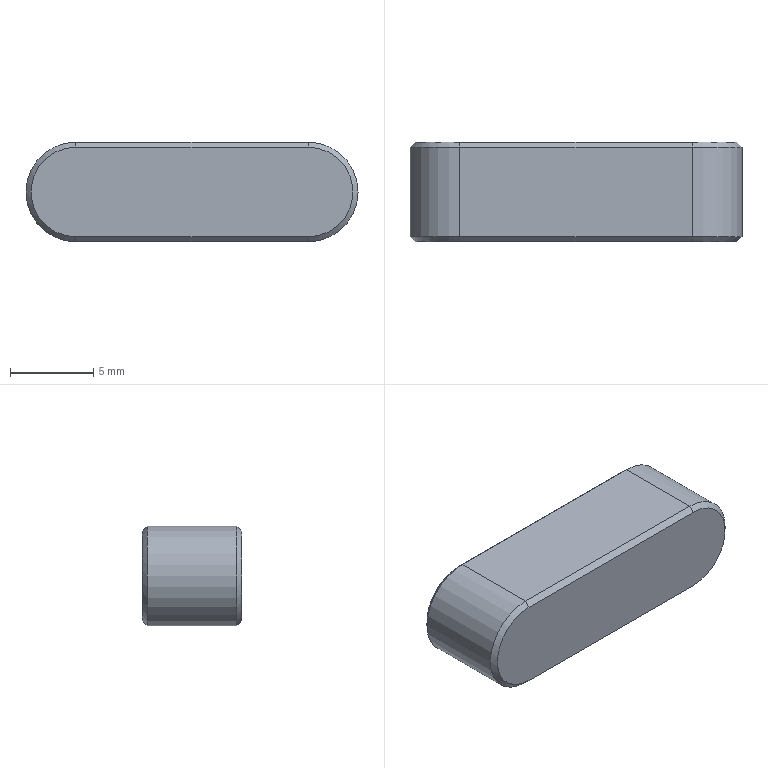Part | NX | features BREP 1 | 1 solid | 14 faces | box 20 x 6 x 6 mm | volume 669.486 mm3 | plane 8 | cone 4 | cylinder 2 | commonest cylinder face diameters 6 x2
STEP:
#1=CARTESIAN_POINT('',(-7.,5.7,3.));
#2=VERTEX_POINT('',#1);
#3=CARTESIAN_POINT('',(-7.,0.3,3.));
#4=VERTEX_POINT('',#3);
#5=CARTESIAN_POINT('',(-7.,6.,3.));
#6=DIRECTION('',(0.,-1.,0.));
#7=VECTOR('',#6,1000.);
#8=LINE('',#5,#7);
#9=EDGE_CURVE('',#2,#4,#8,.T.);
#10=ORIENTED_EDGE('',*,*,#9,.F.);
#11=CARTESIAN_POINT('',(-7.,5.7,-3.));
#12=VERTEX_POINT('',#11);
#13=CARTESIAN_POINT('',(-7.,5.7,0.));
#14=DIRECTION('',(0.,-1.,0.));
#15=DIRECTION('',(0.,0.,1.));
#16=AXIS2_PLACEMENT_3D('',#13,#14,#15);
#17=CIRCLE('',#16,3.);
#18=EDGE_CURVE('',#2,#12,#17,.T.);
#19=ORIENTED_EDGE('',*,*,#18,.T.);
#20=CARTESIAN_POINT('',(-7.,0.3,-3.));
#21=VERTEX_POINT('',#20);
#22=CARTESIAN_POINT('',(-7.,6.,-3.));
#23=DIRECTION('',(0.,-1.,0.));
#24=VECTOR('',#23,1000.);
#25=LINE('',#22,#24);
#26=EDGE_CURVE('',#12,#21,#25,.T.);
#27=ORIENTED_EDGE('',*,*,#26,.T.);
#28=CARTESIAN_POINT('',(-7.,0.3,0.));
#29=DIRECTION('',(0.,1.,0.));
#30=DIRECTION('',(0.,0.,1.));
#31=AXIS2_PLACEMENT_3D('',#28,#29,#30);
#32=CIRCLE('',#31,3.);
#33=EDGE_CURVE('',#21,#4,#32,.T.);
#34=ORIENTED_EDGE('',*,*,#33,.T.);
#35=EDGE_LOOP('',(#10,#19,#27,#34));
#36=FACE_BOUND('',#35,.T.);
#37=CARTESIAN_POINT('',(-7.,6.,0.));
#38=DIRECTION('',(0.,-1.,0.));
#39=DIRECTION('',(0.,0.,1.));
#40=AXIS2_PLACEMENT_3D('',#37,#38,#39);
#41=CYLINDRICAL_SURFACE('',#40,3.);
#42=ADVANCED_FACE('',(#36),#41,.T.);
#43=CARTESIAN_POINT('',(7.,5.7,3.));
#44=VERTEX_POINT('',#43);
#45=CARTESIAN_POINT('',(7.,0.3,3.));
#46=VERTEX_POINT('',#45);
#47=CARTESIAN_POINT('',(7.,6.,3.));
#48=DIRECTION('',(0.,-1.,0.));
#49=VECTOR('',#48,1000.);
#50=LINE('',#47,#49);
#51=EDGE_CURVE('',#44,#46,#50,.T.);
#52=ORIENTED_EDGE('',*,*,#51,.F.);
#53=CARTESIAN_POINT('',(-7.,5.7,3.));
#54=DIRECTION('',(-1.,0.,0.));
#55=VECTOR('',#54,1000.);
#56=LINE('',#53,#55);
#57=EDGE_CURVE('',#44,#2,#56,.T.);
#58=ORIENTED_EDGE('',*,*,#57,.T.);
#59=ORIENTED_EDGE('',*,*,#9,.T.);
#60=CARTESIAN_POINT('',(-7.,0.3,3.));
#61=DIRECTION('',(1.,0.,0.));
#62=VECTOR('',#61,1000.);
#63=LINE('',#60,#62);
#64=EDGE_CURVE('',#4,#46,#63,.T.);
#65=ORIENTED_EDGE('',*,*,#64,.T.);
#66=EDGE_LOOP('',(#52,#58,#59,#65));
#67=FACE_BOUND('',#66,.T.);
#68=CARTESIAN_POINT('',(-7.,6.,3.));
#69=DIRECTION('',(0.,0.,-1.));
#70=DIRECTION('',(1.,0.,0.));
#71=AXIS2_PLACEMENT_3D('',#68,#69,#70);
#72=PLANE('',#71);
#73=ADVANCED_FACE('',(#67),#72,.F.);
#74=CARTESIAN_POINT('',(7.,5.7,-3.));
#75=VERTEX_POINT('',#74);
#76=CARTESIAN_POINT('',(7.,0.3,-3.));
#77=VERTEX_POINT('',#76);
#78=CARTESIAN_POINT('',(7.,6.,-3.));
#79=DIRECTION('',(0.,-1.,0.));
#80=VECTOR('',#79,1000.);
#81=LINE('',#78,#80);
#82=EDGE_CURVE('',#75,#77,#81,.T.);
#83=ORIENTED_EDGE('',*,*,#82,.F.);
#84=CARTESIAN_POINT('',(7.,5.7,0.));
#85=DIRECTION('',(0.,-1.,0.));
#86=DIRECTION('',(0.,0.,1.));
#87=AXIS2_PLACEMENT_3D('',#84,#85,#86);
#88=CIRCLE('',#87,3.);
#89=EDGE_CURVE('',#75,#44,#88,.T.);
#90=ORIENTED_EDGE('',*,*,#89,.T.);
#91=ORIENTED_EDGE('',*,*,#51,.T.);
#92=CARTESIAN_POINT('',(7.,0.3,0.));
#93=DIRECTION('',(0.,1.,0.));
#94=DIRECTION('',(0.,0.,1.));
#95=AXIS2_PLACEMENT_3D('',#92,#93,#94);
#96=CIRCLE('',#95,3.);
#97=EDGE_CURVE('',#46,#77,#96,.T.);
#98=ORIENTED_EDGE('',*,*,#97,.T.);
#99=EDGE_LOOP('',(#83,#90,#91,#98));
#100=FACE_BOUND('',#99,.T.);
#101=CARTESIAN_POINT('',(7.,6.,0.));
#102=DIRECTION('',(0.,-1.,0.));
#103=DIRECTION('',(0.,0.,1.));
#104=AXIS2_PLACEMENT_3D('',#101,#102,#103);
#105=CYLINDRICAL_SURFACE('',#104,3.);
#106=ADVANCED_FACE('',(#100),#105,.T.);
#107=ORIENTED_EDGE('',*,*,#26,.F.);
#108=CARTESIAN_POINT('',(7.,5.7,-3.));
#109=DIRECTION('',(1.,0.,0.));
#110=VECTOR('',#109,1000.);
#111=LINE('',#108,#110);
#112=EDGE_CURVE('',#12,#75,#111,.T.);
#113=ORIENTED_EDGE('',*,*,#112,.T.);
#114=ORIENTED_EDGE('',*,*,#82,.T.);
#115=CARTESIAN_POINT('',(7.,0.3,-3.));
#116=DIRECTION('',(-1.,0.,0.));
#117=VECTOR('',#116,1000.);
#118=LINE('',#115,#117);
#119=EDGE_CURVE('',#77,#21,#118,.T.);
#120=ORIENTED_EDGE('',*,*,#119,.T.);
#121=EDGE_LOOP('',(#107,#113,#114,#120));
#122=FACE_BOUND('',#121,.T.);
#123=CARTESIAN_POINT('',(7.,6.,-3.));
#124=DIRECTION('',(0.,0.,1.));
#125=DIRECTION('',(-1.,0.,0.));
#126=AXIS2_PLACEMENT_3D('',#123,#124,#125);
#127=PLANE('',#126);
#128=ADVANCED_FACE('',(#122),#127,.F.);
#129=CARTESIAN_POINT('',(7.,6.,-2.7));
#130=VERTEX_POINT('',#129);
#131=CARTESIAN_POINT('',(-7.,6.,-2.7));
#132=VERTEX_POINT('',#131);
#133=CARTESIAN_POINT('',(-7.,6.,-2.7));
#134=DIRECTION('',(-1.,0.,0.));
#135=VECTOR('',#134,1000.);
#136=LINE('',#133,#135);
#137=EDGE_CURVE('',#130,#132,#136,.T.);
#138=ORIENTED_EDGE('',*,*,#137,.T.);
#139=CARTESIAN_POINT('',(-7.,6.,2.7));
#140=VERTEX_POINT('',#139);
#141=CARTESIAN_POINT('',(-7.,6.,0.));
#142=DIRECTION('',(0.,1.,0.));
#143=DIRECTION('',(0.,0.,1.));
#144=AXIS2_PLACEMENT_3D('',#141,#142,#143);
#145=CIRCLE('',#144,2.7);
#146=EDGE_CURVE('',#132,#140,#145,.T.);
#147=ORIENTED_EDGE('',*,*,#146,.T.);
#148=CARTESIAN_POINT('',(7.,6.,2.7));
#149=VERTEX_POINT('',#148);
#150=CARTESIAN_POINT('',(7.,6.,2.7));
#151=DIRECTION('',(1.,0.,0.));
#152=VECTOR('',#151,1000.);
#153=LINE('',#150,#152);
#154=EDGE_CURVE('',#140,#149,#153,.T.);
#155=ORIENTED_EDGE('',*,*,#154,.T.);
#156=CARTESIAN_POINT('',(7.,6.,0.));
#157=DIRECTION('',(0.,1.,0.));
#158=DIRECTION('',(0.,0.,1.));
#159=AXIS2_PLACEMENT_3D('',#156,#157,#158);
#160=CIRCLE('',#159,2.7);
#161=EDGE_CURVE('',#149,#130,#160,.T.);
#162=ORIENTED_EDGE('',*,*,#161,.T.);
#163=EDGE_LOOP('',(#138,#147,#155,#162));
#164=FACE_BOUND('',#163,.T.);
#165=CARTESIAN_POINT('',(-7.,6.,0.));
#166=DIRECTION('',(0.,1.,0.));
#167=DIRECTION('',(0.,0.,-1.));
#168=AXIS2_PLACEMENT_3D('',#165,#166,#167);
#169=PLANE('',#168);
#170=ADVANCED_FACE('',(#164),#169,.T.);
#171=CARTESIAN_POINT('',(7.,0.,2.7));
#172=VERTEX_POINT('',#171);
#173=CARTESIAN_POINT('',(-7.,0.,2.7));
#174=VERTEX_POINT('',#173);
#175=CARTESIAN_POINT('',(-7.,0.,2.7));
#176=DIRECTION('',(-1.,0.,0.));
#177=VECTOR('',#176,1000.);
#178=LINE('',#175,#177);
#179=EDGE_CURVE('',#172,#174,#178,.T.);
#180=ORIENTED_EDGE('',*,*,#179,.T.);
#181=CARTESIAN_POINT('',(-7.,0.,-2.7));
#182=VERTEX_POINT('',#181);
#183=CARTESIAN_POINT('',(-7.,0.,0.));
#184=DIRECTION('',(0.,-1.,0.));
#185=DIRECTION('',(0.,0.,1.));
#186=AXIS2_PLACEMENT_3D('',#183,#184,#185);
#187=CIRCLE('',#186,2.7);
#188=EDGE_CURVE('',#174,#182,#187,.T.);
#189=ORIENTED_EDGE('',*,*,#188,.T.);
#190=CARTESIAN_POINT('',(7.,0.,-2.7));
#191=VERTEX_POINT('',#190);
#192=CARTESIAN_POINT('',(-7.,0.,-2.7));
#193=DIRECTION('',(1.,0.,0.));
#194=VECTOR('',#193,1000.);
#195=LINE('',#192,#194);
#196=EDGE_CURVE('',#182,#191,#195,.T.);
#197=ORIENTED_EDGE('',*,*,#196,.T.);
#198=CARTESIAN_POINT('',(7.,0.,0.));
#199=DIRECTION('',(0.,-1.,0.));
#200=DIRECTION('',(0.,0.,1.));
#201=AXIS2_PLACEMENT_3D('',#198,#199,#200);
#202=CIRCLE('',#201,2.7);
#203=EDGE_CURVE('',#191,#172,#202,.T.);
#204=ORIENTED_EDGE('',*,*,#203,.T.);
#205=EDGE_LOOP('',(#180,#189,#197,#204));
#206=FACE_BOUND('',#205,.T.);
#207=CARTESIAN_POINT('',(-7.,0.,0.));
#208=DIRECTION('',(0.,1.,0.));
#209=DIRECTION('',(0.,0.,-1.));
#210=AXIS2_PLACEMENT_3D('',#207,#208,#209);
#211=PLANE('',#210);
#212=ADVANCED_FACE('',(#206),#211,.F.);
#213=CARTESIAN_POINT('',(7.,5.7,3.));
#214=DIRECTION('',(0.,0.7071,-0.7071));
#215=VECTOR('',#214,1000.);
#216=LINE('',#213,#215);
#217=EDGE_CURVE('',#44,#149,#216,.T.);
#218=ORIENTED_EDGE('',*,*,#217,.F.);
#219=ORIENTED_EDGE('',*,*,#89,.F.);
#220=CARTESIAN_POINT('',(7.,6.,-2.7));
#221=DIRECTION('',(0.,-0.7071,-0.7071));
#222=VECTOR('',#221,1000.);
#223=LINE('',#220,#222);
#224=EDGE_CURVE('',#130,#75,#223,.T.);
#225=ORIENTED_EDGE('',*,*,#224,.F.);
#226=ORIENTED_EDGE('',*,*,#161,.F.);
#227=EDGE_LOOP('',(#218,#219,#225,#226));
#228=FACE_BOUND('',#227,.T.);
#229=CARTESIAN_POINT('',(7.,6.,0.));
#230=DIRECTION('',(0.,-1.,0.));
#231=DIRECTION('',(0.,0.,1.));
#232=AXIS2_PLACEMENT_3D('',#229,#230,#231);
#233=CONICAL_SURFACE('',#232,2.7,0.7854);
#234=ADVANCED_FACE('',(#228),#233,.T.);
#235=ORIENTED_EDGE('',*,*,#224,.T.);
#236=ORIENTED_EDGE('',*,*,#112,.F.);
#237=CARTESIAN_POINT('',(-7.,6.,-2.7));
#238=DIRECTION('',(0.,-0.7071,-0.7071));
#239=VECTOR('',#238,1000.);
#240=LINE('',#237,#239);
#241=EDGE_CURVE('',#132,#12,#240,.T.);
#242=ORIENTED_EDGE('',*,*,#241,.F.);
#243=ORIENTED_EDGE('',*,*,#137,.F.);
#244=EDGE_LOOP('',(#235,#236,#242,#243));
#245=FACE_BOUND('',#244,.T.);
#246=CARTESIAN_POINT('',(-7.,6.,-2.7));
#247=DIRECTION('',(0.,0.7071,-0.7071));
#248=DIRECTION('',(-1.,0.,0.));
#249=AXIS2_PLACEMENT_3D('',#246,#247,#248);
#250=PLANE('',#249);
#251=ADVANCED_FACE('',(#245),#250,.T.);
#252=ORIENTED_EDGE('',*,*,#217,.T.);
#253=ORIENTED_EDGE('',*,*,#154,.F.);
#254=CARTESIAN_POINT('',(-7.,5.7,3.));
#255=DIRECTION('',(0.,0.7071,-0.7071));
#256=VECTOR('',#255,1000.);
#257=LINE('',#254,#256);
#258=EDGE_CURVE('',#2,#140,#257,.T.);
#259=ORIENTED_EDGE('',*,*,#258,.F.);
#260=ORIENTED_EDGE('',*,*,#57,.F.);
#261=EDGE_LOOP('',(#252,#253,#259,#260));
#262=FACE_BOUND('',#261,.T.);
#263=CARTESIAN_POINT('',(-7.,6.,2.7));
#264=DIRECTION('',(0.,0.7071,0.7071));
#265=DIRECTION('',(1.,0.,0.));
#266=AXIS2_PLACEMENT_3D('',#263,#264,#265);
#267=PLANE('',#266);
#268=ADVANCED_FACE('',(#262),#267,.T.);
#269=ORIENTED_EDGE('',*,*,#241,.T.);
#270=ORIENTED_EDGE('',*,*,#18,.F.);
#271=ORIENTED_EDGE('',*,*,#258,.T.);
#272=ORIENTED_EDGE('',*,*,#146,.F.);
#273=EDGE_LOOP('',(#269,#270,#271,#272));
#274=FACE_BOUND('',#273,.T.);
#275=CARTESIAN_POINT('',(-7.,6.,0.));
#276=DIRECTION('',(0.,-1.,0.));
#277=DIRECTION('',(0.,0.,1.));
#278=AXIS2_PLACEMENT_3D('',#275,#276,#277);
#279=CONICAL_SURFACE('',#278,2.7,0.7854);
#280=ADVANCED_FACE('',(#274),#279,.T.);
#281=CARTESIAN_POINT('',(7.,0.,2.7));
#282=DIRECTION('',(0.,0.7071,0.7071));
#283=VECTOR('',#282,1000.);
#284=LINE('',#281,#283);
#285=EDGE_CURVE('',#172,#46,#284,.T.);
#286=ORIENTED_EDGE('',*,*,#285,.F.);
#287=ORIENTED_EDGE('',*,*,#203,.F.);
#288=CARTESIAN_POINT('',(7.,0.3,-3.));
#289=DIRECTION('',(0.,-0.7071,0.7071));
#290=VECTOR('',#289,1000.);
#291=LINE('',#288,#290);
#292=EDGE_CURVE('',#77,#191,#291,.T.);
#293=ORIENTED_EDGE('',*,*,#292,.F.);
#294=ORIENTED_EDGE('',*,*,#97,.F.);
#295=EDGE_LOOP('',(#286,#287,#293,#294));
#296=FACE_BOUND('',#295,.T.);
#297=CARTESIAN_POINT('',(7.,0.3,0.));
#298=DIRECTION('',(0.,1.,0.));
#299=DIRECTION('',(0.,0.,-1.));
#300=AXIS2_PLACEMENT_3D('',#297,#298,#299);
#301=CONICAL_SURFACE('',#300,3.,0.7854);
#302=ADVANCED_FACE('',(#296),#301,.T.);
#303=ORIENTED_EDGE('',*,*,#292,.T.);
#304=ORIENTED_EDGE('',*,*,#196,.F.);
#305=CARTESIAN_POINT('',(-7.,0.3,-3.));
#306=DIRECTION('',(0.,-0.7071,0.7071));
#307=VECTOR('',#306,1000.);
#308=LINE('',#305,#307);
#309=EDGE_CURVE('',#21,#182,#308,.T.);
#310=ORIENTED_EDGE('',*,*,#309,.F.);
#311=ORIENTED_EDGE('',*,*,#119,.F.);
#312=EDGE_LOOP('',(#303,#304,#310,#311));
#313=FACE_BOUND('',#312,.T.);
#314=CARTESIAN_POINT('',(7.,0.3,-3.));
#315=DIRECTION('',(0.,0.7071,0.7071));
#316=DIRECTION('',(1.,0.,0.));
#317=AXIS2_PLACEMENT_3D('',#314,#315,#316);
#318=PLANE('',#317);
#319=ADVANCED_FACE('',(#313),#318,.F.);
#320=ORIENTED_EDGE('',*,*,#285,.T.);
#321=ORIENTED_EDGE('',*,*,#64,.F.);
#322=CARTESIAN_POINT('',(-7.,0.,2.7));
#323=DIRECTION('',(0.,0.7071,0.7071));
#324=VECTOR('',#323,1000.);
#325=LINE('',#322,#324);
#326=EDGE_CURVE('',#174,#4,#325,.T.);
#327=ORIENTED_EDGE('',*,*,#326,.F.);
#328=ORIENTED_EDGE('',*,*,#179,.F.);
#329=EDGE_LOOP('',(#320,#321,#327,#328));
#330=FACE_BOUND('',#329,.T.);
#331=CARTESIAN_POINT('',(-7.,0.3,3.));
#332=DIRECTION('',(0.,0.7071,-0.7071));
#333=DIRECTION('',(-1.,0.,0.));
#334=AXIS2_PLACEMENT_3D('',#331,#332,#333);
#335=PLANE('',#334);
#336=ADVANCED_FACE('',(#330),#335,.F.);
#337=ORIENTED_EDGE('',*,*,#309,.T.);
#338=ORIENTED_EDGE('',*,*,#188,.F.);
#339=ORIENTED_EDGE('',*,*,#326,.T.);
#340=ORIENTED_EDGE('',*,*,#33,.F.);
#341=EDGE_LOOP('',(#337,#338,#339,#340));
#342=FACE_BOUND('',#341,.T.);
#343=CARTESIAN_POINT('',(-7.,0.3,0.));
#344=DIRECTION('',(0.,1.,0.));
#345=DIRECTION('',(0.,0.,-1.));
#346=AXIS2_PLACEMENT_3D('',#343,#344,#345);
#347=CONICAL_SURFACE('',#346,3.,0.7854);
#348=ADVANCED_FACE('',(#342),#347,.T.);
#349=CLOSED_SHELL('',(#42,#73,#106,#128,#170,#212,#234,#251,#268,#280,#302,#319,#336,#348));
#350=MANIFOLD_SOLID_BREP('',#349);
#351=(LENGTH_UNIT()NAMED_UNIT(*)SI_UNIT(.MILLI.,.METRE.));
#352=UNCERTAINTY_MEASURE_WITH_UNIT(LENGTH_MEASURE(0.00001),#351,'','');
#353=(NAMED_UNIT(*)PLANE_ANGLE_UNIT()SI_UNIT($,.RADIAN.));
#354=(NAMED_UNIT(*)SI_UNIT($,.STERADIAN.)SOLID_ANGLE_UNIT());
#355=(GEOMETRIC_REPRESENTATION_CONTEXT(3)GLOBAL_UNCERTAINTY_ASSIGNED_CONTEXT((#352))GLOBAL_UNIT_ASSIGNED_CONTEXT((#351,#353,#354))REPRESENTATION_CONTEXT('',''));
#356=ADVANCED_BREP_SHAPE_REPRESENTATION('',(#350),#355);